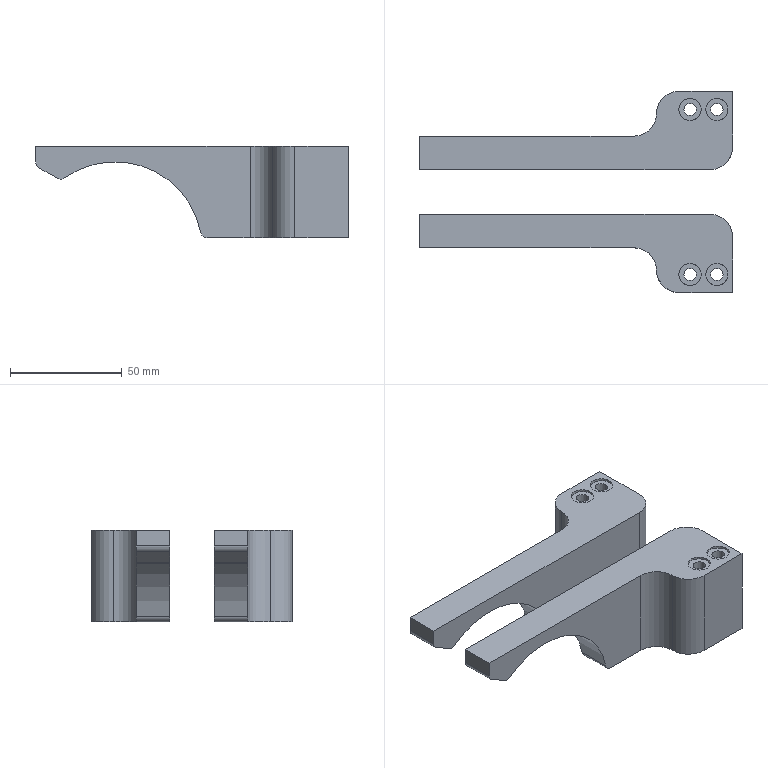Part | 2 solids | 50 faces | box 140 x 90 x 41 mm | volume 149726 mm3 | plane 26 | cylinder 24 | commonest cylinder face diameters 6 x6 20 x6 5.5 x4 10 x4 12.2 x2 78 x2
STEP:
#1=CARTESIAN_POINT('',(-68.5,-52.5,-9.64));
#2=VERTEX_POINT('',#1);
#3=CARTESIAN_POINT('',(-68.5,-37.5,-9.64));
#4=VERTEX_POINT('',#3);
#5=CARTESIAN_POINT('',(-68.5,-72.5,-9.64));
#6=DIRECTION('',(0.,1.,0.));
#7=VECTOR('',#6,1000.);
#8=LINE('',#5,#7);
#9=EDGE_CURVE('',#2,#4,#8,.T.);
#10=ORIENTED_EDGE('',*,*,#9,.F.);
#11=CARTESIAN_POINT('',(-70.,-52.5,-7.041));
#12=VERTEX_POINT('',#11);
#13=CARTESIAN_POINT('',(-67.,-52.5,-7.041));
#14=DIRECTION('',(0.,1.,0.));
#15=DIRECTION('',(-1.,0.,0.));
#16=AXIS2_PLACEMENT_3D('',#13,#14,#15);
#17=CIRCLE('',#16,3.);
#18=EDGE_CURVE('',#2,#12,#17,.T.);
#19=ORIENTED_EDGE('',*,*,#18,.T.);
#20=CARTESIAN_POINT('',(-70.,-37.5,-7.041));
#21=VERTEX_POINT('',#20);
#22=CARTESIAN_POINT('',(-70.,-72.5,-7.041));
#23=DIRECTION('',(0.,1.,0.));
#24=VECTOR('',#23,1000.);
#25=LINE('',#22,#24);
#26=EDGE_CURVE('',#12,#21,#25,.T.);
#27=ORIENTED_EDGE('',*,*,#26,.T.);
#28=CARTESIAN_POINT('',(-67.,-37.5,-7.041));
#29=DIRECTION('',(0.,-1.,0.));
#30=DIRECTION('',(1.,0.,0.));
#31=AXIS2_PLACEMENT_3D('',#28,#29,#30);
#32=CIRCLE('',#31,3.);
#33=EDGE_CURVE('',#21,#4,#32,.T.);
#34=ORIENTED_EDGE('',*,*,#33,.T.);
#35=EDGE_LOOP('',(#10,#19,#27,#34));
#36=FACE_BOUND('',#35,.T.);
#37=CARTESIAN_POINT('',(-67.,-72.5,-7.041));
#38=DIRECTION('',(0.,1.,0.));
#39=DIRECTION('',(-1.,0.,0.));
#40=AXIS2_PLACEMENT_3D('',#37,#38,#39);
#41=CYLINDRICAL_SURFACE('',#40,3.);
#42=ADVANCED_FACE('',(#36),#41,.T.);
#43=CARTESIAN_POINT('',(-60.27,-52.5,-14.391));
#44=VERTEX_POINT('',#43);
#45=CARTESIAN_POINT('',(-60.27,-37.5,-14.391));
#46=VERTEX_POINT('',#45);
#47=CARTESIAN_POINT('',(-60.27,-72.5,-14.391));
#48=DIRECTION('',(0.,1.,0.));
#49=VECTOR('',#48,1000.);
#50=LINE('',#47,#49);
#51=EDGE_CURVE('',#44,#46,#50,.T.);
#52=ORIENTED_EDGE('',*,*,#51,.F.);
#53=CARTESIAN_POINT('',(-68.5,-52.5,-9.64));
#54=DIRECTION('',(-0.866,0.,0.5));
#55=VECTOR('',#54,1000.);
#56=LINE('',#53,#55);
#57=EDGE_CURVE('',#44,#2,#56,.T.);
#58=ORIENTED_EDGE('',*,*,#57,.T.);
#59=ORIENTED_EDGE('',*,*,#9,.T.);
#60=CARTESIAN_POINT('',(-68.5,-37.5,-9.64));
#61=DIRECTION('',(0.866,0.,-0.5));
#62=VECTOR('',#61,1000.);
#63=LINE('',#60,#62);
#64=EDGE_CURVE('',#4,#46,#63,.T.);
#65=ORIENTED_EDGE('',*,*,#64,.T.);
#66=EDGE_LOOP('',(#52,#58,#59,#65));
#67=FACE_BOUND('',#66,.T.);
#68=CARTESIAN_POINT('',(-68.5,-72.5,-9.64));
#69=DIRECTION('',(0.5,0.,0.866));
#70=DIRECTION('',(-0.866,0.,0.5));
#71=AXIS2_PLACEMENT_3D('',#68,#69,#70);
#72=PLANE('',#71);
#73=ADVANCED_FACE('',(#67),#72,.F.);
#74=CARTESIAN_POINT('',(3.886,-52.5,-38.571));
#75=VERTEX_POINT('',#74);
#76=CARTESIAN_POINT('',(3.886,-37.5,-38.571));
#77=VERTEX_POINT('',#76);
#78=CARTESIAN_POINT('',(3.886,-72.5,-38.571));
#79=DIRECTION('',(0.,1.,0.));
#80=VECTOR('',#79,1000.);
#81=LINE('',#78,#80);
#82=EDGE_CURVE('',#75,#77,#81,.T.);
#83=ORIENTED_EDGE('',*,*,#82,.F.);
#84=CARTESIAN_POINT('',(-57.029,-52.5,-14.236));
#85=VERTEX_POINT('',#84);
#86=CARTESIAN_POINT('',(-34.4,-52.5,-46.));
#87=DIRECTION('',(0.,1.,0.));
#88=DIRECTION('',(-1.,0.,0.));
#89=AXIS2_PLACEMENT_3D('',#86,#87,#88);
#90=CIRCLE('',#89,39.);
#91=EDGE_CURVE('',#75,#85,#90,.F.);
#92=ORIENTED_EDGE('',*,*,#91,.T.);
#93=CARTESIAN_POINT('',(-57.029,-37.5,-14.236));
#94=VERTEX_POINT('',#93);
#95=CARTESIAN_POINT('',(-57.029,-72.5,-14.236));
#96=DIRECTION('',(0.,1.,0.));
#97=VECTOR('',#96,1000.);
#98=LINE('',#95,#97);
#99=EDGE_CURVE('',#85,#94,#98,.T.);
#100=ORIENTED_EDGE('',*,*,#99,.T.);
#101=CARTESIAN_POINT('',(-34.4,-37.5,-46.));
#102=DIRECTION('',(0.,1.,0.));
#103=DIRECTION('',(1.,0.,0.));
#104=AXIS2_PLACEMENT_3D('',#101,#102,#103);
#105=CIRCLE('',#104,39.);
#106=EDGE_CURVE('',#94,#77,#105,.T.);
#107=ORIENTED_EDGE('',*,*,#106,.T.);
#108=EDGE_LOOP('',(#83,#92,#100,#107));
#109=FACE_BOUND('',#108,.T.);
#110=CARTESIAN_POINT('',(-34.4,-72.5,-46.));
#111=DIRECTION('',(0.,1.,0.));
#112=DIRECTION('',(-1.,0.,0.));
#113=AXIS2_PLACEMENT_3D('',#110,#111,#112);
#114=CYLINDRICAL_SURFACE('',#113,39.);
#115=ADVANCED_FACE('',(#109),#114,.F.);
#116=ORIENTED_EDGE('',*,*,#99,.F.);
#117=CARTESIAN_POINT('',(-58.77,-52.5,-11.793));
#118=DIRECTION('',(0.,1.,0.));
#119=DIRECTION('',(-1.,0.,0.));
#120=AXIS2_PLACEMENT_3D('',#117,#118,#119);
#121=CIRCLE('',#120,3.);
#122=EDGE_CURVE('',#85,#44,#121,.T.);
#123=ORIENTED_EDGE('',*,*,#122,.T.);
#124=ORIENTED_EDGE('',*,*,#51,.T.);
#125=CARTESIAN_POINT('',(-58.77,-37.5,-11.793));
#126=DIRECTION('',(0.,-1.,0.));
#127=DIRECTION('',(1.,0.,0.));
#128=AXIS2_PLACEMENT_3D('',#125,#126,#127);
#129=CIRCLE('',#128,3.);
#130=EDGE_CURVE('',#46,#94,#129,.T.);
#131=ORIENTED_EDGE('',*,*,#130,.T.);
#132=EDGE_LOOP('',(#116,#123,#124,#131));
#133=FACE_BOUND('',#132,.T.);
#134=CARTESIAN_POINT('',(-58.77,-72.5,-11.793));
#135=DIRECTION('',(0.,1.,0.));
#136=DIRECTION('',(-1.,0.,0.));
#137=AXIS2_PLACEMENT_3D('',#134,#135,#136);
#138=CYLINDRICAL_SURFACE('',#137,3.);
#139=ADVANCED_FACE('',(#133),#138,.T.);
#140=CARTESIAN_POINT('',(6.831,-52.5,-41.));
#141=VERTEX_POINT('',#140);
#142=CARTESIAN_POINT('',(6.831,-37.5,-41.));
#143=VERTEX_POINT('',#142);
#144=CARTESIAN_POINT('',(6.831,-72.5,-41.));
#145=DIRECTION('',(0.,1.,0.));
#146=VECTOR('',#145,1000.);
#147=LINE('',#144,#146);
#148=EDGE_CURVE('',#141,#143,#147,.T.);
#149=ORIENTED_EDGE('',*,*,#148,.F.);
#150=CARTESIAN_POINT('',(6.831,-52.5,-38.));
#151=DIRECTION('',(0.,1.,0.));
#152=DIRECTION('',(-1.,0.,0.));
#153=AXIS2_PLACEMENT_3D('',#150,#151,#152);
#154=CIRCLE('',#153,3.);
#155=EDGE_CURVE('',#141,#75,#154,.T.);
#156=ORIENTED_EDGE('',*,*,#155,.T.);
#157=ORIENTED_EDGE('',*,*,#82,.T.);
#158=CARTESIAN_POINT('',(6.831,-37.5,-38.));
#159=DIRECTION('',(0.,-1.,0.));
#160=DIRECTION('',(1.,0.,0.));
#161=AXIS2_PLACEMENT_3D('',#158,#159,#160);
#162=CIRCLE('',#161,3.);
#163=EDGE_CURVE('',#77,#143,#162,.T.);
#164=ORIENTED_EDGE('',*,*,#163,.T.);
#165=EDGE_LOOP('',(#149,#156,#157,#164));
#166=FACE_BOUND('',#165,.T.);
#167=CARTESIAN_POINT('',(6.831,-72.5,-38.));
#168=DIRECTION('',(0.,1.,0.));
#169=DIRECTION('',(-1.,0.,0.));
#170=AXIS2_PLACEMENT_3D('',#167,#168,#169);
#171=CYLINDRICAL_SURFACE('',#170,3.);
#172=ADVANCED_FACE('',(#166),#171,.T.);
#173=CARTESIAN_POINT('',(36.,-62.5,-41.));
#174=VERTEX_POINT('',#173);
#175=CARTESIAN_POINT('',(46.,-72.5,-41.));
#176=VERTEX_POINT('',#175);
#177=CARTESIAN_POINT('',(46.,-62.5,-41.));
#178=DIRECTION('',(0.,0.,1.));
#179=DIRECTION('',(1.,0.,0.));
#180=AXIS2_PLACEMENT_3D('',#177,#178,#179);
#181=CIRCLE('',#180,10.);
#182=EDGE_CURVE('',#174,#176,#181,.T.);
#183=ORIENTED_EDGE('',*,*,#182,.T.);
#184=CARTESIAN_POINT('',(46.,-72.5,0.));
#185=VERTEX_POINT('',#184);
#186=CARTESIAN_POINT('',(46.,-72.5,0.));
#187=DIRECTION('',(0.,0.,-1.));
#188=VECTOR('',#187,1000.);
#189=LINE('',#186,#188);
#190=EDGE_CURVE('',#185,#176,#189,.T.);
#191=ORIENTED_EDGE('',*,*,#190,.F.);
#192=CARTESIAN_POINT('',(36.,-62.5,0.));
#193=VERTEX_POINT('',#192);
#194=CARTESIAN_POINT('',(46.,-62.5,0.));
#195=DIRECTION('',(0.,0.,1.));
#196=DIRECTION('',(1.,0.,0.));
#197=AXIS2_PLACEMENT_3D('',#194,#195,#196);
#198=CIRCLE('',#197,10.);
#199=EDGE_CURVE('',#193,#185,#198,.T.);
#200=ORIENTED_EDGE('',*,*,#199,.F.);
#201=CARTESIAN_POINT('',(36.,-62.5,0.));
#202=DIRECTION('',(0.,0.,-1.));
#203=VECTOR('',#202,1000.);
#204=LINE('',#201,#203);
#205=EDGE_CURVE('',#193,#174,#204,.T.);
#206=ORIENTED_EDGE('',*,*,#205,.T.);
#207=EDGE_LOOP('',(#183,#191,#200,#206));
#208=FACE_BOUND('',#207,.T.);
#209=CARTESIAN_POINT('',(46.,-62.5,0.));
#210=DIRECTION('',(0.,0.,-1.));
#211=DIRECTION('',(1.,0.,0.));
#212=AXIS2_PLACEMENT_3D('',#209,#210,#211);
#213=CYLINDRICAL_SURFACE('',#212,10.);
#214=ADVANCED_FACE('',(#208),#213,.T.);
#215=CARTESIAN_POINT('',(26.,-52.5,-41.));
#216=VERTEX_POINT('',#215);
#217=CARTESIAN_POINT('',(26.,-62.5,-41.));
#218=DIRECTION('',(0.,0.,1.));
#219=DIRECTION('',(0.,-1.,0.));
#220=AXIS2_PLACEMENT_3D('',#217,#218,#219);
#221=CIRCLE('',#220,10.);
#222=EDGE_CURVE('',#216,#174,#221,.F.);
#223=ORIENTED_EDGE('',*,*,#222,.T.);
#224=ORIENTED_EDGE('',*,*,#205,.F.);
#225=CARTESIAN_POINT('',(26.,-52.5,0.));
#226=VERTEX_POINT('',#225);
#227=CARTESIAN_POINT('',(26.,-62.5,0.));
#228=DIRECTION('',(0.,0.,-1.));
#229=DIRECTION('',(0.,1.,0.));
#230=AXIS2_PLACEMENT_3D('',#227,#228,#229);
#231=CIRCLE('',#230,10.);
#232=EDGE_CURVE('',#226,#193,#231,.T.);
#233=ORIENTED_EDGE('',*,*,#232,.F.);
#234=CARTESIAN_POINT('',(26.,-52.5,0.));
#235=DIRECTION('',(0.,0.,-1.));
#236=VECTOR('',#235,1000.);
#237=LINE('',#234,#236);
#238=EDGE_CURVE('',#226,#216,#237,.T.);
#239=ORIENTED_EDGE('',*,*,#238,.T.);
#240=EDGE_LOOP('',(#223,#224,#233,#239));
#241=FACE_BOUND('',#240,.T.);
#242=CARTESIAN_POINT('',(26.,-62.5,0.));
#243=DIRECTION('',(0.,0.,-1.));
#244=DIRECTION('',(1.,0.,0.));
#245=AXIS2_PLACEMENT_3D('',#242,#243,#244);
#246=CYLINDRICAL_SURFACE('',#245,10.);
#247=ADVANCED_FACE('',(#241),#246,.F.);
#248=ORIENTED_EDGE('',*,*,#155,.F.);
#249=CARTESIAN_POINT('',(-60.27,-52.5,-41.));
#250=DIRECTION('',(1.,0.,0.));
#251=VECTOR('',#250,1000.);
#252=LINE('',#249,#251);
#253=EDGE_CURVE('',#141,#216,#252,.T.);
#254=ORIENTED_EDGE('',*,*,#253,.T.);
#255=ORIENTED_EDGE('',*,*,#238,.F.);
#256=CARTESIAN_POINT('',(-70.,-52.5,0.));
#257=VERTEX_POINT('',#256);
#258=CARTESIAN_POINT('',(-57.029,-52.5,0.));
#259=DIRECTION('',(1.,0.,0.));
#260=VECTOR('',#259,1000.);
#261=LINE('',#258,#260);
#262=EDGE_CURVE('',#257,#226,#261,.T.);
#263=ORIENTED_EDGE('',*,*,#262,.F.);
#264=CARTESIAN_POINT('',(-70.,-52.5,0.));
#265=DIRECTION('',(0.,0.,-1.));
#266=VECTOR('',#265,1000.);
#267=LINE('',#264,#266);
#268=EDGE_CURVE('',#257,#12,#267,.T.);
#269=ORIENTED_EDGE('',*,*,#268,.T.);
#270=ORIENTED_EDGE('',*,*,#18,.F.);
#271=ORIENTED_EDGE('',*,*,#57,.F.);
#272=ORIENTED_EDGE('',*,*,#122,.F.);
#273=ORIENTED_EDGE('',*,*,#91,.F.);
#274=EDGE_LOOP('',(#248,#254,#255,#263,#269,#270,#271,#272,#273));
#275=FACE_BOUND('',#274,.T.);
#276=CARTESIAN_POINT('',(-60.27,-52.5,0.));
#277=DIRECTION('',(0.,1.,0.));
#278=DIRECTION('',(0.,0.,1.));
#279=AXIS2_PLACEMENT_3D('',#276,#277,#278);
#280=PLANE('',#279);
#281=ADVANCED_FACE('',(#275),#280,.F.);
#282=CARTESIAN_POINT('',(70.,-47.5,-41.));
#283=VERTEX_POINT('',#282);
#284=CARTESIAN_POINT('',(60.,-37.5,-41.));
#285=VERTEX_POINT('',#284);
#286=CARTESIAN_POINT('',(60.,-47.5,-41.));
#287=DIRECTION('',(0.,0.,1.));
#288=DIRECTION('',(1.,0.,0.));
#289=AXIS2_PLACEMENT_3D('',#286,#287,#288);
#290=CIRCLE('',#289,10.);
#291=EDGE_CURVE('',#283,#285,#290,.T.);
#292=ORIENTED_EDGE('',*,*,#291,.T.);
#293=CARTESIAN_POINT('',(60.,-37.5,0.));
#294=VERTEX_POINT('',#293);
#295=CARTESIAN_POINT('',(60.,-37.5,0.));
#296=DIRECTION('',(0.,0.,-1.));
#297=VECTOR('',#296,1000.);
#298=LINE('',#295,#297);
#299=EDGE_CURVE('',#294,#285,#298,.T.);
#300=ORIENTED_EDGE('',*,*,#299,.F.);
#301=CARTESIAN_POINT('',(70.,-47.5,0.));
#302=VERTEX_POINT('',#301);
#303=CARTESIAN_POINT('',(60.,-47.5,0.));
#304=DIRECTION('',(0.,0.,1.));
#305=DIRECTION('',(1.,0.,0.));
#306=AXIS2_PLACEMENT_3D('',#303,#304,#305);
#307=CIRCLE('',#306,10.);
#308=EDGE_CURVE('',#302,#294,#307,.T.);
#309=ORIENTED_EDGE('',*,*,#308,.F.);
#310=CARTESIAN_POINT('',(70.,-47.5,0.));
#311=DIRECTION('',(0.,0.,-1.));
#312=VECTOR('',#311,1000.);
#313=LINE('',#310,#312);
#314=EDGE_CURVE('',#302,#283,#313,.T.);
#315=ORIENTED_EDGE('',*,*,#314,.T.);
#316=EDGE_LOOP('',(#292,#300,#309,#315));
#317=FACE_BOUND('',#316,.T.);
#318=CARTESIAN_POINT('',(60.,-47.5,0.));
#319=DIRECTION('',(0.,0.,-1.));
#320=DIRECTION('',(1.,0.,0.));
#321=AXIS2_PLACEMENT_3D('',#318,#319,#320);
#322=CYLINDRICAL_SURFACE('',#321,10.);
#323=ADVANCED_FACE('',(#317),#322,.T.);
#324=CARTESIAN_POINT('',(65.753,-64.4,-1.));
#325=VERTEX_POINT('',#324);
#326=CARTESIAN_POINT('',(63.003,-64.4,-1.));
#327=DIRECTION('',(0.,0.,-1.));
#328=DIRECTION('',(1.,0.,0.));
#329=AXIS2_PLACEMENT_3D('',#326,#327,#328);
#330=CIRCLE('',#329,2.75);
#331=EDGE_CURVE('',#325,#325,#330,.F.);
#332=ORIENTED_EDGE('',*,*,#331,.T.);
#333=EDGE_LOOP('',(#332));
#334=FACE_BOUND('',#333,.T.);
#335=CARTESIAN_POINT('',(60.253,-64.4,-25.8));
#336=VERTEX_POINT('',#335);
#337=CARTESIAN_POINT('',(63.003,-64.4,-25.8));
#338=DIRECTION('',(0.,0.,1.));
#339=DIRECTION('',(-1.,0.,0.));
#340=AXIS2_PLACEMENT_3D('',#337,#338,#339);
#341=CIRCLE('',#340,2.75);
#342=EDGE_CURVE('',#336,#336,#341,.F.);
#343=ORIENTED_EDGE('',*,*,#342,.T.);
#344=EDGE_LOOP('',(#343));
#345=FACE_BOUND('',#344,.T.);
#346=CARTESIAN_POINT('',(63.003,-64.4,0.));
#347=DIRECTION('',(0.,0.,-1.));
#348=DIRECTION('',(1.,0.,0.));
#349=AXIS2_PLACEMENT_3D('',#346,#347,#348);
#350=CYLINDRICAL_SURFACE('',#349,2.75);
#351=ADVANCED_FACE('',(#334,#345),#350,.F.);
#352=CARTESIAN_POINT('',(44.9,-58.3,-41.));
#353=VERTEX_POINT('',#352);
#354=CARTESIAN_POINT('',(44.9,-70.5,-41.));
#355=VERTEX_POINT('',#354);
#356=CARTESIAN_POINT('',(44.9,-64.4,-41.));
#357=DIRECTION('',(0.,0.,1.));
#358=DIRECTION('',(0.,-1.,0.));
#359=AXIS2_PLACEMENT_3D('',#356,#357,#358);
#360=CIRCLE('',#359,6.1);
#361=EDGE_CURVE('',#353,#355,#360,.T.);
#362=ORIENTED_EDGE('',*,*,#361,.F.);
#363=CARTESIAN_POINT('',(44.9,-58.3,-25.8));
#364=VERTEX_POINT('',#363);
#365=CARTESIAN_POINT('',(44.9,-58.3,-25.8));
#366=DIRECTION('',(0.,0.,-1.));
#367=VECTOR('',#366,1000.);
#368=LINE('',#365,#367);
#369=EDGE_CURVE('',#353,#364,#368,.F.);
#370=ORIENTED_EDGE('',*,*,#369,.T.);
#371=CARTESIAN_POINT('',(44.9,-70.5,-25.8));
#372=VERTEX_POINT('',#371);
#373=CARTESIAN_POINT('',(44.9,-64.4,-25.8));
#374=DIRECTION('',(0.,0.,1.));
#375=DIRECTION('',(1.,0.,0.));
#376=AXIS2_PLACEMENT_3D('',#373,#374,#375);
#377=CIRCLE('',#376,6.1);
#378=EDGE_CURVE('',#372,#364,#377,.F.);
#379=ORIENTED_EDGE('',*,*,#378,.F.);
#380=CARTESIAN_POINT('',(44.9,-70.5,-25.8));
#381=DIRECTION('',(0.,0.,-1.));
#382=VECTOR('',#381,1000.);
#383=LINE('',#380,#382);
#384=EDGE_CURVE('',#355,#372,#383,.F.);
#385=ORIENTED_EDGE('',*,*,#384,.F.);
#386=EDGE_LOOP('',(#362,#370,#379,#385));
#387=FACE_BOUND('',#386,.T.);
#388=CARTESIAN_POINT('',(44.9,-64.4,-25.8));
#389=DIRECTION('',(0.,0.,-1.));
#390=DIRECTION('',(1.,0.,0.));
#391=AXIS2_PLACEMENT_3D('',#388,#389,#390);
#392=CYLINDRICAL_SURFACE('',#391,6.1);
#393=ADVANCED_FACE('',(#387),#392,.F.);
#394=CARTESIAN_POINT('',(70.,-70.5,-41.));
#395=VERTEX_POINT('',#394);
#396=CARTESIAN_POINT('',(44.9,-70.5,-41.));
#397=DIRECTION('',(1.,0.,0.));
#398=VECTOR('',#397,1000.);
#399=LINE('',#396,#398);
#400=EDGE_CURVE('',#355,#395,#399,.T.);
#401=ORIENTED_EDGE('',*,*,#400,.F.);
#402=ORIENTED_EDGE('',*,*,#384,.T.);
#403=CARTESIAN_POINT('',(70.,-70.5,-25.8));
#404=VERTEX_POINT('',#403);
#405=CARTESIAN_POINT('',(44.9,-70.5,-25.8));
#406=DIRECTION('',(1.,0.,0.));
#407=VECTOR('',#406,1000.);
#408=LINE('',#405,#407);
#409=EDGE_CURVE('',#404,#372,#408,.F.);
#410=ORIENTED_EDGE('',*,*,#409,.F.);
#411=CARTESIAN_POINT('',(70.,-70.5,-25.8));
#412=DIRECTION('',(0.,0.,-1.));
#413=VECTOR('',#412,1000.);
#414=LINE('',#411,#413);
#415=EDGE_CURVE('',#404,#395,#414,.T.);
#416=ORIENTED_EDGE('',*,*,#415,.T.);
#417=EDGE_LOOP('',(#401,#402,#410,#416));
#418=FACE_BOUND('',#417,.T.);
#419=CARTESIAN_POINT('',(44.9,-70.5,-25.8));
#420=DIRECTION('',(0.,1.,0.));
#421=DIRECTION('',(0.,0.,1.));
#422=AXIS2_PLACEMENT_3D('',#419,#420,#421);
#423=PLANE('',#422);
#424=ADVANCED_FACE('',(#418),#423,.T.);
#425=CARTESIAN_POINT('',(70.,-58.3,-41.));
#426=VERTEX_POINT('',#425);
#427=CARTESIAN_POINT('',(70.,-58.3,-41.));
#428=DIRECTION('',(-1.,0.,0.));
#429=VECTOR('',#428,1000.);
#430=LINE('',#427,#429);
#431=EDGE_CURVE('',#426,#353,#430,.T.);
#432=ORIENTED_EDGE('',*,*,#431,.F.);
#433=CARTESIAN_POINT('',(70.,-58.3,-25.8));
#434=VERTEX_POINT('',#433);
#435=CARTESIAN_POINT('',(70.,-58.3,-25.8));
#436=DIRECTION('',(0.,0.,-1.));
#437=VECTOR('',#436,1000.);
#438=LINE('',#435,#437);
#439=EDGE_CURVE('',#434,#426,#438,.T.);
#440=ORIENTED_EDGE('',*,*,#439,.F.);
#441=CARTESIAN_POINT('',(70.,-58.3,-25.8));
#442=DIRECTION('',(-1.,0.,0.));
#443=VECTOR('',#442,1000.);
#444=LINE('',#441,#443);
#445=EDGE_CURVE('',#364,#434,#444,.F.);
#446=ORIENTED_EDGE('',*,*,#445,.F.);
#447=ORIENTED_EDGE('',*,*,#369,.F.);
#448=EDGE_LOOP('',(#432,#440,#446,#447));
#449=FACE_BOUND('',#448,.T.);
#450=CARTESIAN_POINT('',(70.,-58.3,-25.8));
#451=DIRECTION('',(0.,-1.,0.));
#452=DIRECTION('',(0.,0.,-1.));
#453=AXIS2_PLACEMENT_3D('',#450,#451,#452);
#454=PLANE('',#453);
#455=ADVANCED_FACE('',(#449),#454,.T.);
#456=CARTESIAN_POINT('',(53.753,-64.4,-1.));
#457=VERTEX_POINT('',#456);
#458=CARTESIAN_POINT('',(51.003,-64.4,-1.));
#459=DIRECTION('',(0.,0.,-1.));
#460=DIRECTION('',(1.,0.,0.));
#461=AXIS2_PLACEMENT_3D('',#458,#459,#460);
#462=CIRCLE('',#461,2.75);
#463=EDGE_CURVE('',#457,#457,#462,.F.);
#464=ORIENTED_EDGE('',*,*,#463,.T.);
#465=EDGE_LOOP('',(#464));
#466=FACE_BOUND('',#465,.T.);
#467=CARTESIAN_POINT('',(48.253,-64.4,-25.8));
#468=VERTEX_POINT('',#467);
#469=CARTESIAN_POINT('',(51.003,-64.4,-25.8));
#470=DIRECTION('',(0.,0.,1.));
#471=DIRECTION('',(-1.,0.,0.));
#472=AXIS2_PLACEMENT_3D('',#469,#470,#471);
#473=CIRCLE('',#472,2.75);
#474=EDGE_CURVE('',#468,#468,#473,.F.);
#475=ORIENTED_EDGE('',*,*,#474,.T.);
#476=EDGE_LOOP('',(#475));
#477=FACE_BOUND('',#476,.T.);
#478=CARTESIAN_POINT('',(51.003,-64.4,0.));
#479=DIRECTION('',(0.,0.,-1.));
#480=DIRECTION('',(1.,0.,0.));
#481=AXIS2_PLACEMENT_3D('',#478,#479,#480);
#482=CYLINDRICAL_SURFACE('',#481,2.75);
#483=ADVANCED_FACE('',(#466,#477),#482,.F.);
#484=ORIENTED_EDGE('',*,*,#474,.F.);
#485=EDGE_LOOP('',(#484));
#486=FACE_BOUND('',#485,.T.);
#487=ORIENTED_EDGE('',*,*,#445,.T.);
#488=CARTESIAN_POINT('',(70.,-72.5,-25.8));
#489=DIRECTION('',(0.,1.,0.));
#490=VECTOR('',#489,1000.);
#491=LINE('',#488,#490);
#492=EDGE_CURVE('',#404,#434,#491,.T.);
#493=ORIENTED_EDGE('',*,*,#492,.F.);
#494=ORIENTED_EDGE('',*,*,#409,.T.);
#495=ORIENTED_EDGE('',*,*,#378,.T.);
#496=EDGE_LOOP('',(#487,#493,#494,#495));
#497=FACE_BOUND('',#496,.T.);
#498=ORIENTED_EDGE('',*,*,#342,.F.);
#499=EDGE_LOOP('',(#498));
#500=FACE_BOUND('',#499,.T.);
#501=CARTESIAN_POINT('',(44.9,-64.4,-25.8));
#502=DIRECTION('',(0.,0.,1.));
#503=DIRECTION('',(-1.,0.,0.));
#504=AXIS2_PLACEMENT_3D('',#501,#502,#503);
#505=PLANE('',#504);
#506=ADVANCED_FACE('',(#486,#497,#500),#505,.F.);
#507=CARTESIAN_POINT('',(68.003,-64.4,-1.));
#508=VERTEX_POINT('',#507);
#509=CARTESIAN_POINT('',(63.003,-64.4,-1.));
#510=DIRECTION('',(0.,0.,-1.));
#511=DIRECTION('',(1.,0.,0.));
#512=AXIS2_PLACEMENT_3D('',#509,#510,#511);
#513=CIRCLE('',#512,5.);
#514=EDGE_CURVE('',#508,#508,#513,.F.);
#515=ORIENTED_EDGE('',*,*,#514,.T.);
#516=EDGE_LOOP('',(#515));
#517=FACE_BOUND('',#516,.T.);
#518=ORIENTED_EDGE('',*,*,#331,.F.);
#519=EDGE_LOOP('',(#518));
#520=FACE_BOUND('',#519,.T.);
#521=CARTESIAN_POINT('',(63.003,-64.4,-1.));
#522=DIRECTION('',(0.,0.,-1.));
#523=DIRECTION('',(1.,0.,0.));
#524=AXIS2_PLACEMENT_3D('',#521,#522,#523);
#525=PLANE('',#524);
#526=ADVANCED_FACE('',(#517,#520),#525,.F.);
#527=ORIENTED_EDGE('',*,*,#514,.F.);
#528=EDGE_LOOP('',(#527));
#529=FACE_BOUND('',#528,.T.);
#530=CARTESIAN_POINT('',(63.003,-59.4,0.));
#531=VERTEX_POINT('',#530);
#532=CARTESIAN_POINT('',(63.003,-64.4,0.));
#533=DIRECTION('',(0.,0.,-1.));
#534=DIRECTION('',(0.,1.,0.));
#535=AXIS2_PLACEMENT_3D('',#532,#533,#534);
#536=CIRCLE('',#535,5.);
#537=EDGE_CURVE('',#531,#531,#536,.T.);
#538=ORIENTED_EDGE('',*,*,#537,.F.);
#539=EDGE_LOOP('',(#538));
#540=FACE_BOUND('',#539,.T.);
#541=CARTESIAN_POINT('',(63.003,-64.4,-1.));
#542=DIRECTION('',(0.,0.,1.));
#543=DIRECTION('',(-1.,0.,0.));
#544=AXIS2_PLACEMENT_3D('',#541,#542,#543);
#545=CYLINDRICAL_SURFACE('',#544,5.);
#546=ADVANCED_FACE('',(#529,#540),#545,.F.);
#547=CARTESIAN_POINT('',(56.003,-64.4,-1.));
#548=VERTEX_POINT('',#547);
#549=CARTESIAN_POINT('',(51.003,-64.4,-1.));
#550=DIRECTION('',(0.,0.,-1.));
#551=DIRECTION('',(1.,0.,0.));
#552=AXIS2_PLACEMENT_3D('',#549,#550,#551);
#553=CIRCLE('',#552,5.);
#554=EDGE_CURVE('',#548,#548,#553,.F.);
#555=ORIENTED_EDGE('',*,*,#554,.T.);
#556=EDGE_LOOP('',(#555));
#557=FACE_BOUND('',#556,.T.);
#558=ORIENTED_EDGE('',*,*,#463,.F.);
#559=EDGE_LOOP('',(#558));
#560=FACE_BOUND('',#559,.T.);
#561=CARTESIAN_POINT('',(51.003,-64.4,-1.));
#562=DIRECTION('',(0.,0.,-1.));
#563=DIRECTION('',(1.,0.,0.));
#564=AXIS2_PLACEMENT_3D('',#561,#562,#563);
#565=PLANE('',#564);
#566=ADVANCED_FACE('',(#557,#560),#565,.F.);
#567=ORIENTED_EDGE('',*,*,#554,.F.);
#568=EDGE_LOOP('',(#567));
#569=FACE_BOUND('',#568,.T.);
#570=CARTESIAN_POINT('',(51.003,-59.4,0.));
#571=VERTEX_POINT('',#570);
#572=CARTESIAN_POINT('',(51.003,-64.4,0.));
#573=DIRECTION('',(0.,0.,-1.));
#574=DIRECTION('',(0.,1.,0.));
#575=AXIS2_PLACEMENT_3D('',#572,#573,#574);
#576=CIRCLE('',#575,5.);
#577=EDGE_CURVE('',#571,#571,#576,.T.);
#578=ORIENTED_EDGE('',*,*,#577,.F.);
#579=EDGE_LOOP('',(#578));
#580=FACE_BOUND('',#579,.T.);
#581=CARTESIAN_POINT('',(51.003,-64.4,-1.));
#582=DIRECTION('',(0.,0.,1.));
#583=DIRECTION('',(-1.,0.,0.));
#584=AXIS2_PLACEMENT_3D('',#581,#582,#583);
#585=CYLINDRICAL_SURFACE('',#584,5.);
#586=ADVANCED_FACE('',(#569,#580),#585,.F.);
#587=ORIENTED_EDGE('',*,*,#314,.F.);
#588=CARTESIAN_POINT('',(70.,-72.5,0.));
#589=VERTEX_POINT('',#588);
#590=CARTESIAN_POINT('',(70.,-72.5,0.));
#591=DIRECTION('',(0.,1.,0.));
#592=VECTOR('',#591,1000.);
#593=LINE('',#590,#592);
#594=EDGE_CURVE('',#589,#302,#593,.T.);
#595=ORIENTED_EDGE('',*,*,#594,.F.);
#596=CARTESIAN_POINT('',(70.,-72.5,-41.));
#597=VERTEX_POINT('',#596);
#598=CARTESIAN_POINT('',(70.,-72.5,-41.));
#599=DIRECTION('',(0.,0.,1.));
#600=VECTOR('',#599,1000.);
#601=LINE('',#598,#600);
#602=EDGE_CURVE('',#589,#597,#601,.F.);
#603=ORIENTED_EDGE('',*,*,#602,.T.);
#604=CARTESIAN_POINT('',(70.,-72.5,-41.));
#605=DIRECTION('',(0.,1.,0.));
#606=VECTOR('',#605,1000.);
#607=LINE('',#604,#606);
#608=EDGE_CURVE('',#597,#395,#607,.T.);
#609=ORIENTED_EDGE('',*,*,#608,.T.);
#610=ORIENTED_EDGE('',*,*,#415,.F.);
#611=ORIENTED_EDGE('',*,*,#492,.T.);
#612=ORIENTED_EDGE('',*,*,#439,.T.);
#613=CARTESIAN_POINT('',(70.,-72.5,-41.));
#614=DIRECTION('',(0.,1.,0.));
#615=VECTOR('',#614,1000.);
#616=LINE('',#613,#615);
#617=EDGE_CURVE('',#426,#283,#616,.T.);
#618=ORIENTED_EDGE('',*,*,#617,.T.);
#619=EDGE_LOOP('',(#587,#595,#603,#609,#610,#611,#612,#618));
#620=FACE_BOUND('',#619,.T.);
#621=CARTESIAN_POINT('',(70.,-72.5,-41.));
#622=DIRECTION('',(-1.,0.,0.));
#623=DIRECTION('',(0.,-1.,0.));
#624=AXIS2_PLACEMENT_3D('',#621,#622,#623);
#625=PLANE('',#624);
#626=ADVANCED_FACE('',(#620),#625,.F.);
#627=ORIENTED_EDGE('',*,*,#617,.F.);
#628=ORIENTED_EDGE('',*,*,#431,.T.);
#629=ORIENTED_EDGE('',*,*,#361,.T.);
#630=ORIENTED_EDGE('',*,*,#400,.T.);
#631=ORIENTED_EDGE('',*,*,#608,.F.);
#632=CARTESIAN_POINT('',(6.831,-72.5,-41.));
#633=DIRECTION('',(1.,0.,0.));
#634=VECTOR('',#633,1000.);
#635=LINE('',#632,#634);
#636=EDGE_CURVE('',#176,#597,#635,.T.);
#637=ORIENTED_EDGE('',*,*,#636,.F.);
#638=ORIENTED_EDGE('',*,*,#182,.F.);
#639=ORIENTED_EDGE('',*,*,#222,.F.);
#640=ORIENTED_EDGE('',*,*,#253,.F.);
#641=ORIENTED_EDGE('',*,*,#148,.T.);
#642=CARTESIAN_POINT('',(46.,-37.5,-41.));
#643=DIRECTION('',(1.,0.,0.));
#644=VECTOR('',#643,1000.);
#645=LINE('',#642,#644);
#646=EDGE_CURVE('',#285,#143,#645,.F.);
#647=ORIENTED_EDGE('',*,*,#646,.F.);
#648=ORIENTED_EDGE('',*,*,#291,.F.);
#649=EDGE_LOOP('',(#627,#628,#629,#630,#631,#637,#638,#639,#640,#641,#647,#648));
#650=FACE_BOUND('',#649,.T.);
#651=CARTESIAN_POINT('',(46.,-72.5,-41.));
#652=DIRECTION('',(0.,0.,1.));
#653=DIRECTION('',(0.,-1.,0.));
#654=AXIS2_PLACEMENT_3D('',#651,#652,#653);
#655=PLANE('',#654);
#656=ADVANCED_FACE('',(#650),#655,.F.);
#657=ORIENTED_EDGE('',*,*,#577,.T.);
#658=EDGE_LOOP('',(#657));
#659=FACE_BOUND('',#658,.T.);
#660=ORIENTED_EDGE('',*,*,#537,.T.);
#661=EDGE_LOOP('',(#660));
#662=FACE_BOUND('',#661,.T.);
#663=CARTESIAN_POINT('',(-70.,-37.5,0.));
#664=VERTEX_POINT('',#663);
#665=CARTESIAN_POINT('',(-70.,-72.5,0.));
#666=DIRECTION('',(0.,1.,0.));
#667=VECTOR('',#666,1000.);
#668=LINE('',#665,#667);
#669=EDGE_CURVE('',#664,#257,#668,.F.);
#670=ORIENTED_EDGE('',*,*,#669,.T.);
#671=ORIENTED_EDGE('',*,*,#262,.T.);
#672=ORIENTED_EDGE('',*,*,#232,.T.);
#673=ORIENTED_EDGE('',*,*,#199,.T.);
#674=CARTESIAN_POINT('',(70.,-72.5,0.));
#675=DIRECTION('',(-1.,0.,0.));
#676=VECTOR('',#675,1000.);
#677=LINE('',#674,#676);
#678=EDGE_CURVE('',#185,#589,#677,.F.);
#679=ORIENTED_EDGE('',*,*,#678,.T.);
#680=ORIENTED_EDGE('',*,*,#594,.T.);
#681=ORIENTED_EDGE('',*,*,#308,.T.);
#682=CARTESIAN_POINT('',(-60.,-37.5,0.));
#683=DIRECTION('',(-1.,0.,0.));
#684=VECTOR('',#683,1000.);
#685=LINE('',#682,#684);
#686=EDGE_CURVE('',#294,#664,#685,.T.);
#687=ORIENTED_EDGE('',*,*,#686,.T.);
#688=EDGE_LOOP('',(#670,#671,#672,#673,#679,#680,#681,#687));
#689=FACE_BOUND('',#688,.T.);
#690=CARTESIAN_POINT('',(-60.,-72.5,0.));
#691=DIRECTION('',(0.,0.,-1.));
#692=DIRECTION('',(0.,1.,0.));
#693=AXIS2_PLACEMENT_3D('',#690,#691,#692);
#694=PLANE('',#693);
#695=ADVANCED_FACE('',(#659,#662,#689),#694,.F.);
#696=ORIENTED_EDGE('',*,*,#686,.F.);
#697=ORIENTED_EDGE('',*,*,#299,.T.);
#698=ORIENTED_EDGE('',*,*,#646,.T.);
#699=ORIENTED_EDGE('',*,*,#163,.F.);
#700=ORIENTED_EDGE('',*,*,#106,.F.);
#701=ORIENTED_EDGE('',*,*,#130,.F.);
#702=ORIENTED_EDGE('',*,*,#64,.F.);
#703=ORIENTED_EDGE('',*,*,#33,.F.);
#704=CARTESIAN_POINT('',(-70.,-37.5,0.));
#705=DIRECTION('',(0.,0.,-1.));
#706=VECTOR('',#705,1000.);
#707=LINE('',#704,#706);
#708=EDGE_CURVE('',#664,#21,#707,.T.);
#709=ORIENTED_EDGE('',*,*,#708,.F.);
#710=EDGE_LOOP('',(#696,#697,#698,#699,#700,#701,#702,#703,#709));
#711=FACE_BOUND('',#710,.T.);
#712=CARTESIAN_POINT('',(-34.4,-37.5,-46.));
#713=DIRECTION('',(0.,1.,0.));
#714=DIRECTION('',(-1.,0.,0.));
#715=AXIS2_PLACEMENT_3D('',#712,#713,#714);
#716=PLANE('',#715);
#717=ADVANCED_FACE('',(#711),#716,.T.);
#718=ORIENTED_EDGE('',*,*,#678,.F.);
#719=ORIENTED_EDGE('',*,*,#190,.T.);
#720=ORIENTED_EDGE('',*,*,#636,.T.);
#721=ORIENTED_EDGE('',*,*,#602,.F.);
#722=EDGE_LOOP('',(#718,#719,#720,#721));
#723=FACE_BOUND('',#722,.T.);
#724=CARTESIAN_POINT('',(-34.4,-72.5,-46.));
#725=DIRECTION('',(0.,1.,0.));
#726=DIRECTION('',(-1.,0.,0.));
#727=AXIS2_PLACEMENT_3D('',#724,#725,#726);
#728=PLANE('',#727);
#729=ADVANCED_FACE('',(#723),#728,.F.);
#730=ORIENTED_EDGE('',*,*,#268,.F.);
#731=ORIENTED_EDGE('',*,*,#669,.F.);
#732=ORIENTED_EDGE('',*,*,#708,.T.);
#733=ORIENTED_EDGE('',*,*,#26,.F.);
#734=EDGE_LOOP('',(#730,#731,#732,#733));
#735=FACE_BOUND('',#734,.T.);
#736=CARTESIAN_POINT('',(-70.,-72.5,0.));
#737=DIRECTION('',(1.,0.,0.));
#738=DIRECTION('',(0.,1.,0.));
#739=AXIS2_PLACEMENT_3D('',#736,#737,#738);
#740=PLANE('',#739);
#741=ADVANCED_FACE('',(#735),#740,.F.);
#742=CLOSED_SHELL('',(#42,#73,#115,#139,#172,#214,#247,#281,#323,#351,#393,#424,#455,#483,#506,#526,#546,#566,#586,#626,#656,#695,#717,#729,#741));
#743=MANIFOLD_SOLID_BREP('',#742);
#744=CARTESIAN_POINT('',(36.,7.5,-41.));
#745=VERTEX_POINT('',#744);
#746=CARTESIAN_POINT('',(46.,17.5,-41.));
#747=VERTEX_POINT('',#746);
#748=CARTESIAN_POINT('',(46.,7.5,-41.));
#749=DIRECTION('',(0.,0.,-1.));
#750=DIRECTION('',(1.,0.,0.));
#751=AXIS2_PLACEMENT_3D('',#748,#749,#750);
#752=CIRCLE('',#751,10.);
#753=EDGE_CURVE('',#745,#747,#752,.T.);
#754=ORIENTED_EDGE('',*,*,#753,.F.);
#755=CARTESIAN_POINT('',(36.,7.5,0.));
#756=VERTEX_POINT('',#755);
#757=CARTESIAN_POINT('',(36.,7.5,0.));
#758=DIRECTION('',(0.,0.,-1.));
#759=VECTOR('',#758,1000.);
#760=LINE('',#757,#759);
#761=EDGE_CURVE('',#756,#745,#760,.T.);
#762=ORIENTED_EDGE('',*,*,#761,.F.);
#763=CARTESIAN_POINT('',(46.,17.5,0.));
#764=VERTEX_POINT('',#763);
#765=CARTESIAN_POINT('',(46.,7.5,0.));
#766=DIRECTION('',(0.,0.,-1.));
#767=DIRECTION('',(1.,0.,0.));
#768=AXIS2_PLACEMENT_3D('',#765,#766,#767);
#769=CIRCLE('',#768,10.);
#770=EDGE_CURVE('',#756,#764,#769,.T.);
#771=ORIENTED_EDGE('',*,*,#770,.T.);
#772=CARTESIAN_POINT('',(46.,17.5,0.));
#773=DIRECTION('',(0.,0.,-1.));
#774=VECTOR('',#773,1000.);
#775=LINE('',#772,#774);
#776=EDGE_CURVE('',#764,#747,#775,.T.);
#777=ORIENTED_EDGE('',*,*,#776,.T.);
#778=EDGE_LOOP('',(#754,#762,#771,#777));
#779=FACE_BOUND('',#778,.T.);
#780=CARTESIAN_POINT('',(46.,7.5,0.));
#781=DIRECTION('',(0.,0.,-1.));
#782=DIRECTION('',(1.,0.,0.));
#783=AXIS2_PLACEMENT_3D('',#780,#781,#782);
#784=CYLINDRICAL_SURFACE('',#783,10.);
#785=ADVANCED_FACE('',(#779),#784,.T.);
#786=CARTESIAN_POINT('',(26.,-2.5,-41.));
#787=VERTEX_POINT('',#786);
#788=CARTESIAN_POINT('',(26.,7.5,-41.));
#789=DIRECTION('',(0.,0.,-1.));
#790=DIRECTION('',(0.,1.,0.));
#791=AXIS2_PLACEMENT_3D('',#788,#789,#790);
#792=CIRCLE('',#791,10.);
#793=EDGE_CURVE('',#787,#745,#792,.F.);
#794=ORIENTED_EDGE('',*,*,#793,.F.);
#795=CARTESIAN_POINT('',(26.,-2.5,0.));
#796=VERTEX_POINT('',#795);
#797=CARTESIAN_POINT('',(26.,-2.5,0.));
#798=DIRECTION('',(0.,0.,-1.));
#799=VECTOR('',#798,1000.);
#800=LINE('',#797,#799);
#801=EDGE_CURVE('',#796,#787,#800,.T.);
#802=ORIENTED_EDGE('',*,*,#801,.F.);
#803=CARTESIAN_POINT('',(26.,7.5,0.));
#804=DIRECTION('',(0.,0.,1.));
#805=DIRECTION('',(0.,-1.,0.));
#806=AXIS2_PLACEMENT_3D('',#803,#804,#805);
#807=CIRCLE('',#806,10.);
#808=EDGE_CURVE('',#796,#756,#807,.T.);
#809=ORIENTED_EDGE('',*,*,#808,.T.);
#810=ORIENTED_EDGE('',*,*,#761,.T.);
#811=EDGE_LOOP('',(#794,#802,#809,#810));
#812=FACE_BOUND('',#811,.T.);
#813=CARTESIAN_POINT('',(26.,7.5,0.));
#814=DIRECTION('',(0.,0.,-1.));
#815=DIRECTION('',(1.,0.,0.));
#816=AXIS2_PLACEMENT_3D('',#813,#814,#815);
#817=CYLINDRICAL_SURFACE('',#816,10.);
#818=ADVANCED_FACE('',(#812),#817,.F.);
#819=CARTESIAN_POINT('',(6.831,-2.5,-41.));
#820=VERTEX_POINT('',#819);
#821=CARTESIAN_POINT('',(3.886,-2.5,-38.571));
#822=VERTEX_POINT('',#821);
#823=CARTESIAN_POINT('',(6.831,-2.5,-38.));
#824=DIRECTION('',(0.,1.,0.));
#825=DIRECTION('',(-1.,0.,0.));
#826=AXIS2_PLACEMENT_3D('',#823,#824,#825);
#827=CIRCLE('',#826,3.);
#828=EDGE_CURVE('',#820,#822,#827,.T.);
#829=ORIENTED_EDGE('',*,*,#828,.T.);
#830=CARTESIAN_POINT('',(-57.029,-2.5,-14.236));
#831=VERTEX_POINT('',#830);
#832=CARTESIAN_POINT('',(-34.4,-2.5,-46.));
#833=DIRECTION('',(0.,1.,0.));
#834=DIRECTION('',(-1.,0.,0.));
#835=AXIS2_PLACEMENT_3D('',#832,#833,#834);
#836=CIRCLE('',#835,39.);
#837=EDGE_CURVE('',#822,#831,#836,.F.);
#838=ORIENTED_EDGE('',*,*,#837,.T.);
#839=CARTESIAN_POINT('',(-60.27,-2.5,-14.391));
#840=VERTEX_POINT('',#839);
#841=CARTESIAN_POINT('',(-58.77,-2.5,-11.793));
#842=DIRECTION('',(0.,1.,0.));
#843=DIRECTION('',(-1.,0.,0.));
#844=AXIS2_PLACEMENT_3D('',#841,#842,#843);
#845=CIRCLE('',#844,3.);
#846=EDGE_CURVE('',#831,#840,#845,.T.);
#847=ORIENTED_EDGE('',*,*,#846,.T.);
#848=CARTESIAN_POINT('',(-68.5,-2.5,-9.64));
#849=VERTEX_POINT('',#848);
#850=CARTESIAN_POINT('',(-68.5,-2.5,-9.64));
#851=DIRECTION('',(-0.866,0.,0.5));
#852=VECTOR('',#851,1000.);
#853=LINE('',#850,#852);
#854=EDGE_CURVE('',#840,#849,#853,.T.);
#855=ORIENTED_EDGE('',*,*,#854,.T.);
#856=CARTESIAN_POINT('',(-70.,-2.5,-7.041));
#857=VERTEX_POINT('',#856);
#858=CARTESIAN_POINT('',(-67.,-2.5,-7.041));
#859=DIRECTION('',(0.,1.,0.));
#860=DIRECTION('',(-1.,0.,0.));
#861=AXIS2_PLACEMENT_3D('',#858,#859,#860);
#862=CIRCLE('',#861,3.);
#863=EDGE_CURVE('',#849,#857,#862,.T.);
#864=ORIENTED_EDGE('',*,*,#863,.T.);
#865=CARTESIAN_POINT('',(-70.,-2.5,0.));
#866=VERTEX_POINT('',#865);
#867=CARTESIAN_POINT('',(-70.,-2.5,0.));
#868=DIRECTION('',(0.,0.,-1.));
#869=VECTOR('',#868,1000.);
#870=LINE('',#867,#869);
#871=EDGE_CURVE('',#866,#857,#870,.T.);
#872=ORIENTED_EDGE('',*,*,#871,.F.);
#873=CARTESIAN_POINT('',(-57.029,-2.5,0.));
#874=DIRECTION('',(1.,0.,0.));
#875=VECTOR('',#874,1000.);
#876=LINE('',#873,#875);
#877=EDGE_CURVE('',#866,#796,#876,.T.);
#878=ORIENTED_EDGE('',*,*,#877,.T.);
#879=ORIENTED_EDGE('',*,*,#801,.T.);
#880=CARTESIAN_POINT('',(-60.27,-2.5,-41.));
#881=DIRECTION('',(1.,0.,0.));
#882=VECTOR('',#881,1000.);
#883=LINE('',#880,#882);
#884=EDGE_CURVE('',#820,#787,#883,.T.);
#885=ORIENTED_EDGE('',*,*,#884,.F.);
#886=EDGE_LOOP('',(#829,#838,#847,#855,#864,#872,#878,#879,#885));
#887=FACE_BOUND('',#886,.T.);
#888=CARTESIAN_POINT('',(-60.27,-2.5,0.));
#889=DIRECTION('',(0.,-1.,0.));
#890=DIRECTION('',(0.,0.,1.));
#891=AXIS2_PLACEMENT_3D('',#888,#889,#890);
#892=PLANE('',#891);
#893=ADVANCED_FACE('',(#887),#892,.F.);
#894=CARTESIAN_POINT('',(-68.5,-17.5,-9.64));
#895=VERTEX_POINT('',#894);
#896=CARTESIAN_POINT('',(-68.5,17.5,-9.64));
#897=DIRECTION('',(0.,-1.,0.));
#898=VECTOR('',#897,1000.);
#899=LINE('',#896,#898);
#900=EDGE_CURVE('',#849,#895,#899,.T.);
#901=ORIENTED_EDGE('',*,*,#900,.T.);
#902=CARTESIAN_POINT('',(-70.,-17.5,-7.041));
#903=VERTEX_POINT('',#902);
#904=CARTESIAN_POINT('',(-67.,-17.5,-7.041));
#905=DIRECTION('',(0.,-1.,0.));
#906=DIRECTION('',(1.,0.,0.));
#907=AXIS2_PLACEMENT_3D('',#904,#905,#906);
#908=CIRCLE('',#907,3.);
#909=EDGE_CURVE('',#903,#895,#908,.T.);
#910=ORIENTED_EDGE('',*,*,#909,.F.);
#911=CARTESIAN_POINT('',(-70.,17.5,-7.041));
#912=DIRECTION('',(0.,-1.,0.));
#913=VECTOR('',#912,1000.);
#914=LINE('',#911,#913);
#915=EDGE_CURVE('',#857,#903,#914,.T.);
#916=ORIENTED_EDGE('',*,*,#915,.F.);
#917=ORIENTED_EDGE('',*,*,#863,.F.);
#918=EDGE_LOOP('',(#901,#910,#916,#917));
#919=FACE_BOUND('',#918,.T.);
#920=CARTESIAN_POINT('',(-67.,17.5,-7.041));
#921=DIRECTION('',(0.,-1.,0.));
#922=DIRECTION('',(-1.,0.,0.));
#923=AXIS2_PLACEMENT_3D('',#920,#921,#922);
#924=CYLINDRICAL_SURFACE('',#923,3.);
#925=ADVANCED_FACE('',(#919),#924,.T.);
#926=CARTESIAN_POINT('',(-60.27,-17.5,-14.391));
#927=VERTEX_POINT('',#926);
#928=CARTESIAN_POINT('',(-60.27,17.5,-14.391));
#929=DIRECTION('',(0.,-1.,0.));
#930=VECTOR('',#929,1000.);
#931=LINE('',#928,#930);
#932=EDGE_CURVE('',#840,#927,#931,.T.);
#933=ORIENTED_EDGE('',*,*,#932,.T.);
#934=CARTESIAN_POINT('',(-68.5,-17.5,-9.64));
#935=DIRECTION('',(0.866,0.,-0.5));
#936=VECTOR('',#935,1000.);
#937=LINE('',#934,#936);
#938=EDGE_CURVE('',#895,#927,#937,.T.);
#939=ORIENTED_EDGE('',*,*,#938,.F.);
#940=ORIENTED_EDGE('',*,*,#900,.F.);
#941=ORIENTED_EDGE('',*,*,#854,.F.);
#942=EDGE_LOOP('',(#933,#939,#940,#941));
#943=FACE_BOUND('',#942,.T.);
#944=CARTESIAN_POINT('',(-68.5,17.5,-9.64));
#945=DIRECTION('',(0.5,0.,0.866));
#946=DIRECTION('',(-0.866,0.,0.5));
#947=AXIS2_PLACEMENT_3D('',#944,#945,#946);
#948=PLANE('',#947);
#949=ADVANCED_FACE('',(#943),#948,.F.);
#950=CARTESIAN_POINT('',(3.886,-17.5,-38.571));
#951=VERTEX_POINT('',#950);
#952=CARTESIAN_POINT('',(3.886,17.5,-38.571));
#953=DIRECTION('',(0.,-1.,0.));
#954=VECTOR('',#953,1000.);
#955=LINE('',#952,#954);
#956=EDGE_CURVE('',#822,#951,#955,.T.);
#957=ORIENTED_EDGE('',*,*,#956,.T.);
#958=CARTESIAN_POINT('',(-57.029,-17.5,-14.236));
#959=VERTEX_POINT('',#958);
#960=CARTESIAN_POINT('',(-34.4,-17.5,-46.));
#961=DIRECTION('',(0.,1.,0.));
#962=DIRECTION('',(1.,0.,0.));
#963=AXIS2_PLACEMENT_3D('',#960,#961,#962);
#964=CIRCLE('',#963,39.);
#965=EDGE_CURVE('',#959,#951,#964,.T.);
#966=ORIENTED_EDGE('',*,*,#965,.F.);
#967=CARTESIAN_POINT('',(-57.029,17.5,-14.236));
#968=DIRECTION('',(0.,-1.,0.));
#969=VECTOR('',#968,1000.);
#970=LINE('',#967,#969);
#971=EDGE_CURVE('',#831,#959,#970,.T.);
#972=ORIENTED_EDGE('',*,*,#971,.F.);
#973=ORIENTED_EDGE('',*,*,#837,.F.);
#974=EDGE_LOOP('',(#957,#966,#972,#973));
#975=FACE_BOUND('',#974,.T.);
#976=CARTESIAN_POINT('',(-34.4,17.5,-46.));
#977=DIRECTION('',(0.,-1.,0.));
#978=DIRECTION('',(-1.,0.,0.));
#979=AXIS2_PLACEMENT_3D('',#976,#977,#978);
#980=CYLINDRICAL_SURFACE('',#979,39.);
#981=ADVANCED_FACE('',(#975),#980,.F.);
#982=ORIENTED_EDGE('',*,*,#971,.T.);
#983=CARTESIAN_POINT('',(-58.77,-17.5,-11.793));
#984=DIRECTION('',(0.,-1.,0.));
#985=DIRECTION('',(1.,0.,0.));
#986=AXIS2_PLACEMENT_3D('',#983,#984,#985);
#987=CIRCLE('',#986,3.);
#988=EDGE_CURVE('',#927,#959,#987,.T.);
#989=ORIENTED_EDGE('',*,*,#988,.F.);
#990=ORIENTED_EDGE('',*,*,#932,.F.);
#991=ORIENTED_EDGE('',*,*,#846,.F.);
#992=EDGE_LOOP('',(#982,#989,#990,#991));
#993=FACE_BOUND('',#992,.T.);
#994=CARTESIAN_POINT('',(-58.77,17.5,-11.793));
#995=DIRECTION('',(0.,-1.,0.));
#996=DIRECTION('',(-1.,0.,0.));
#997=AXIS2_PLACEMENT_3D('',#994,#995,#996);
#998=CYLINDRICAL_SURFACE('',#997,3.);
#999=ADVANCED_FACE('',(#993),#998,.T.);
#1000=CARTESIAN_POINT('',(6.831,-17.5,-41.));
#1001=VERTEX_POINT('',#1000);
#1002=CARTESIAN_POINT('',(6.831,17.5,-41.));
#1003=DIRECTION('',(0.,-1.,0.));
#1004=VECTOR('',#1003,1000.);
#1005=LINE('',#1002,#1004);
#1006=EDGE_CURVE('',#820,#1001,#1005,.T.);
#1007=ORIENTED_EDGE('',*,*,#1006,.T.);
#1008=CARTESIAN_POINT('',(6.831,-17.5,-38.));
#1009=DIRECTION('',(0.,-1.,0.));
#1010=DIRECTION('',(1.,0.,0.));
#1011=AXIS2_PLACEMENT_3D('',#1008,#1009,#1010);
#1012=CIRCLE('',#1011,3.);
#1013=EDGE_CURVE('',#951,#1001,#1012,.T.);
#1014=ORIENTED_EDGE('',*,*,#1013,.F.);
#1015=ORIENTED_EDGE('',*,*,#956,.F.);
#1016=ORIENTED_EDGE('',*,*,#828,.F.);
#1017=EDGE_LOOP('',(#1007,#1014,#1015,#1016));
#1018=FACE_BOUND('',#1017,.T.);
#1019=CARTESIAN_POINT('',(6.831,17.5,-38.));
#1020=DIRECTION('',(0.,-1.,0.));
#1021=DIRECTION('',(-1.,0.,0.));
#1022=AXIS2_PLACEMENT_3D('',#1019,#1020,#1021);
#1023=CYLINDRICAL_SURFACE('',#1022,3.);
#1024=ADVANCED_FACE('',(#1018),#1023,.T.);
#1025=CARTESIAN_POINT('',(60.,-17.5,0.));
#1026=VERTEX_POINT('',#1025);
#1027=CARTESIAN_POINT('',(-70.,-17.5,0.));
#1028=VERTEX_POINT('',#1027);
#1029=CARTESIAN_POINT('',(-60.,-17.5,0.));
#1030=DIRECTION('',(-1.,0.,0.));
#1031=VECTOR('',#1030,1000.);
#1032=LINE('',#1029,#1031);
#1033=EDGE_CURVE('',#1026,#1028,#1032,.T.);
#1034=ORIENTED_EDGE('',*,*,#1033,.T.);
#1035=CARTESIAN_POINT('',(-70.,-17.5,0.));
#1036=DIRECTION('',(0.,0.,-1.));
#1037=VECTOR('',#1036,1000.);
#1038=LINE('',#1035,#1037);
#1039=EDGE_CURVE('',#1028,#903,#1038,.T.);
#1040=ORIENTED_EDGE('',*,*,#1039,.T.);
#1041=ORIENTED_EDGE('',*,*,#909,.T.);
#1042=ORIENTED_EDGE('',*,*,#938,.T.);
#1043=ORIENTED_EDGE('',*,*,#988,.T.);
#1044=ORIENTED_EDGE('',*,*,#965,.T.);
#1045=ORIENTED_EDGE('',*,*,#1013,.T.);
#1046=CARTESIAN_POINT('',(60.,-17.5,-41.));
#1047=VERTEX_POINT('',#1046);
#1048=CARTESIAN_POINT('',(46.,-17.5,-41.));
#1049=DIRECTION('',(1.,0.,0.));
#1050=VECTOR('',#1049,1000.);
#1051=LINE('',#1048,#1050);
#1052=EDGE_CURVE('',#1047,#1001,#1051,.F.);
#1053=ORIENTED_EDGE('',*,*,#1052,.F.);
#1054=CARTESIAN_POINT('',(60.,-17.5,0.));
#1055=DIRECTION('',(0.,0.,-1.));
#1056=VECTOR('',#1055,1000.);
#1057=LINE('',#1054,#1056);
#1058=EDGE_CURVE('',#1026,#1047,#1057,.T.);
#1059=ORIENTED_EDGE('',*,*,#1058,.F.);
#1060=EDGE_LOOP('',(#1034,#1040,#1041,#1042,#1043,#1044,#1045,#1053,#1059));
#1061=FACE_BOUND('',#1060,.T.);
#1062=CARTESIAN_POINT('',(-34.4,-17.5,-46.));
#1063=DIRECTION('',(0.,-1.,0.));
#1064=DIRECTION('',(-1.,0.,0.));
#1065=AXIS2_PLACEMENT_3D('',#1062,#1063,#1064);
#1066=PLANE('',#1065);
#1067=ADVANCED_FACE('',(#1061),#1066,.T.);
#1068=CARTESIAN_POINT('',(51.003,4.4,0.));
#1069=VERTEX_POINT('',#1068);
#1070=CARTESIAN_POINT('',(51.003,9.4,0.));
#1071=DIRECTION('',(0.,0.,1.));
#1072=DIRECTION('',(0.,-1.,0.));
#1073=AXIS2_PLACEMENT_3D('',#1070,#1071,#1072);
#1074=CIRCLE('',#1073,5.);
#1075=EDGE_CURVE('',#1069,#1069,#1074,.T.);
#1076=ORIENTED_EDGE('',*,*,#1075,.F.);
#1077=EDGE_LOOP('',(#1076));
#1078=FACE_BOUND('',#1077,.T.);
#1079=CARTESIAN_POINT('',(63.003,4.4,0.));
#1080=VERTEX_POINT('',#1079);
#1081=CARTESIAN_POINT('',(63.003,9.4,0.));
#1082=DIRECTION('',(0.,0.,1.));
#1083=DIRECTION('',(0.,-1.,0.));
#1084=AXIS2_PLACEMENT_3D('',#1081,#1082,#1083);
#1085=CIRCLE('',#1084,5.);
#1086=EDGE_CURVE('',#1080,#1080,#1085,.T.);
#1087=ORIENTED_EDGE('',*,*,#1086,.F.);
#1088=EDGE_LOOP('',(#1087));
#1089=FACE_BOUND('',#1088,.T.);
#1090=CARTESIAN_POINT('',(-70.,17.5,0.));
#1091=DIRECTION('',(0.,-1.,0.));
#1092=VECTOR('',#1091,1000.);
#1093=LINE('',#1090,#1092);
#1094=EDGE_CURVE('',#1028,#866,#1093,.F.);
#1095=ORIENTED_EDGE('',*,*,#1094,.F.);
#1096=ORIENTED_EDGE('',*,*,#1033,.F.);
#1097=CARTESIAN_POINT('',(70.,-7.5,0.));
#1098=VERTEX_POINT('',#1097);
#1099=CARTESIAN_POINT('',(60.,-7.5,0.));
#1100=DIRECTION('',(0.,0.,-1.));
#1101=DIRECTION('',(1.,0.,0.));
#1102=AXIS2_PLACEMENT_3D('',#1099,#1100,#1101);
#1103=CIRCLE('',#1102,10.);
#1104=EDGE_CURVE('',#1098,#1026,#1103,.T.);
#1105=ORIENTED_EDGE('',*,*,#1104,.F.);
#1106=CARTESIAN_POINT('',(70.,17.5,0.));
#1107=VERTEX_POINT('',#1106);
#1108=CARTESIAN_POINT('',(70.,17.5,0.));
#1109=DIRECTION('',(0.,-1.,0.));
#1110=VECTOR('',#1109,1000.);
#1111=LINE('',#1108,#1110);
#1112=EDGE_CURVE('',#1107,#1098,#1111,.T.);
#1113=ORIENTED_EDGE('',*,*,#1112,.F.);
#1114=CARTESIAN_POINT('',(70.,17.5,0.));
#1115=DIRECTION('',(-1.,0.,0.));
#1116=VECTOR('',#1115,1000.);
#1117=LINE('',#1114,#1116);
#1118=EDGE_CURVE('',#764,#1107,#1117,.F.);
#1119=ORIENTED_EDGE('',*,*,#1118,.F.);
#1120=ORIENTED_EDGE('',*,*,#770,.F.);
#1121=ORIENTED_EDGE('',*,*,#808,.F.);
#1122=ORIENTED_EDGE('',*,*,#877,.F.);
#1123=EDGE_LOOP('',(#1095,#1096,#1105,#1113,#1119,#1120,#1121,#1122));
#1124=FACE_BOUND('',#1123,.T.);
#1125=CARTESIAN_POINT('',(-60.,17.5,0.));
#1126=DIRECTION('',(0.,0.,-1.));
#1127=DIRECTION('',(0.,-1.,0.));
#1128=AXIS2_PLACEMENT_3D('',#1125,#1126,#1127);
#1129=PLANE('',#1128);
#1130=ADVANCED_FACE('',(#1078,#1089,#1124),#1129,.F.);
#1131=CARTESIAN_POINT('',(65.753,9.4,-1.));
#1132=VERTEX_POINT('',#1131);
#1133=CARTESIAN_POINT('',(63.003,9.4,-1.));
#1134=DIRECTION('',(0.,0.,1.));
#1135=DIRECTION('',(1.,0.,0.));
#1136=AXIS2_PLACEMENT_3D('',#1133,#1134,#1135);
#1137=CIRCLE('',#1136,2.75);
#1138=EDGE_CURVE('',#1132,#1132,#1137,.F.);
#1139=ORIENTED_EDGE('',*,*,#1138,.F.);
#1140=EDGE_LOOP('',(#1139));
#1141=FACE_BOUND('',#1140,.T.);
#1142=CARTESIAN_POINT('',(60.253,9.4,-25.8));
#1143=VERTEX_POINT('',#1142);
#1144=CARTESIAN_POINT('',(63.003,9.4,-25.8));
#1145=DIRECTION('',(0.,0.,-1.));
#1146=DIRECTION('',(-1.,0.,0.));
#1147=AXIS2_PLACEMENT_3D('',#1144,#1145,#1146);
#1148=CIRCLE('',#1147,2.75);
#1149=EDGE_CURVE('',#1143,#1143,#1148,.F.);
#1150=ORIENTED_EDGE('',*,*,#1149,.F.);
#1151=EDGE_LOOP('',(#1150));
#1152=FACE_BOUND('',#1151,.T.);
#1153=CARTESIAN_POINT('',(63.003,9.4,0.));
#1154=DIRECTION('',(0.,0.,-1.));
#1155=DIRECTION('',(1.,0.,0.));
#1156=AXIS2_PLACEMENT_3D('',#1153,#1154,#1155);
#1157=CYLINDRICAL_SURFACE('',#1156,2.75);
#1158=ADVANCED_FACE('',(#1141,#1152),#1157,.F.);
#1159=CARTESIAN_POINT('',(44.9,3.3,-41.));
#1160=VERTEX_POINT('',#1159);
#1161=CARTESIAN_POINT('',(44.9,15.5,-41.));
#1162=VERTEX_POINT('',#1161);
#1163=CARTESIAN_POINT('',(44.9,9.4,-41.));
#1164=DIRECTION('',(0.,0.,-1.));
#1165=DIRECTION('',(0.,1.,0.));
#1166=AXIS2_PLACEMENT_3D('',#1163,#1164,#1165);
#1167=CIRCLE('',#1166,6.1);
#1168=EDGE_CURVE('',#1160,#1162,#1167,.T.);
#1169=ORIENTED_EDGE('',*,*,#1168,.T.);
#1170=CARTESIAN_POINT('',(44.9,15.5,-25.8));
#1171=VERTEX_POINT('',#1170);
#1172=CARTESIAN_POINT('',(44.9,15.5,-25.8));
#1173=DIRECTION('',(0.,0.,-1.));
#1174=VECTOR('',#1173,1000.);
#1175=LINE('',#1172,#1174);
#1176=EDGE_CURVE('',#1162,#1171,#1175,.F.);
#1177=ORIENTED_EDGE('',*,*,#1176,.T.);
#1178=CARTESIAN_POINT('',(44.9,3.3,-25.8));
#1179=VERTEX_POINT('',#1178);
#1180=CARTESIAN_POINT('',(44.9,9.4,-25.8));
#1181=DIRECTION('',(0.,0.,-1.));
#1182=DIRECTION('',(1.,0.,0.));
#1183=AXIS2_PLACEMENT_3D('',#1180,#1181,#1182);
#1184=CIRCLE('',#1183,6.1);
#1185=EDGE_CURVE('',#1171,#1179,#1184,.F.);
#1186=ORIENTED_EDGE('',*,*,#1185,.T.);
#1187=CARTESIAN_POINT('',(44.9,3.3,-25.8));
#1188=DIRECTION('',(0.,0.,-1.));
#1189=VECTOR('',#1188,1000.);
#1190=LINE('',#1187,#1189);
#1191=EDGE_CURVE('',#1160,#1179,#1190,.F.);
#1192=ORIENTED_EDGE('',*,*,#1191,.F.);
#1193=EDGE_LOOP('',(#1169,#1177,#1186,#1192));
#1194=FACE_BOUND('',#1193,.T.);
#1195=CARTESIAN_POINT('',(44.9,9.4,-25.8));
#1196=DIRECTION('',(0.,0.,-1.));
#1197=DIRECTION('',(1.,0.,0.));
#1198=AXIS2_PLACEMENT_3D('',#1195,#1196,#1197);
#1199=CYLINDRICAL_SURFACE('',#1198,6.1);
#1200=ADVANCED_FACE('',(#1194),#1199,.F.);
#1201=CARTESIAN_POINT('',(70.,15.5,-41.));
#1202=VERTEX_POINT('',#1201);
#1203=CARTESIAN_POINT('',(44.9,15.5,-41.));
#1204=DIRECTION('',(1.,0.,0.));
#1205=VECTOR('',#1204,1000.);
#1206=LINE('',#1203,#1205);
#1207=EDGE_CURVE('',#1162,#1202,#1206,.T.);
#1208=ORIENTED_EDGE('',*,*,#1207,.T.);
#1209=CARTESIAN_POINT('',(70.,15.5,-25.8));
#1210=VERTEX_POINT('',#1209);
#1211=CARTESIAN_POINT('',(70.,15.5,-25.8));
#1212=DIRECTION('',(0.,0.,-1.));
#1213=VECTOR('',#1212,1000.);
#1214=LINE('',#1211,#1213);
#1215=EDGE_CURVE('',#1210,#1202,#1214,.T.);
#1216=ORIENTED_EDGE('',*,*,#1215,.F.);
#1217=CARTESIAN_POINT('',(44.9,15.5,-25.8));
#1218=DIRECTION('',(1.,0.,0.));
#1219=VECTOR('',#1218,1000.);
#1220=LINE('',#1217,#1219);
#1221=EDGE_CURVE('',#1210,#1171,#1220,.F.);
#1222=ORIENTED_EDGE('',*,*,#1221,.T.);
#1223=ORIENTED_EDGE('',*,*,#1176,.F.);
#1224=EDGE_LOOP('',(#1208,#1216,#1222,#1223));
#1225=FACE_BOUND('',#1224,.T.);
#1226=CARTESIAN_POINT('',(44.9,15.5,-25.8));
#1227=DIRECTION('',(0.,-1.,0.));
#1228=DIRECTION('',(0.,0.,1.));
#1229=AXIS2_PLACEMENT_3D('',#1226,#1227,#1228);
#1230=PLANE('',#1229);
#1231=ADVANCED_FACE('',(#1225),#1230,.T.);
#1232=CARTESIAN_POINT('',(70.,3.3,-41.));
#1233=VERTEX_POINT('',#1232);
#1234=CARTESIAN_POINT('',(70.,3.3,-41.));
#1235=DIRECTION('',(-1.,0.,0.));
#1236=VECTOR('',#1235,1000.);
#1237=LINE('',#1234,#1236);
#1238=EDGE_CURVE('',#1233,#1160,#1237,.T.);
#1239=ORIENTED_EDGE('',*,*,#1238,.T.);
#1240=ORIENTED_EDGE('',*,*,#1191,.T.);
#1241=CARTESIAN_POINT('',(70.,3.3,-25.8));
#1242=VERTEX_POINT('',#1241);
#1243=CARTESIAN_POINT('',(70.,3.3,-25.8));
#1244=DIRECTION('',(-1.,0.,0.));
#1245=VECTOR('',#1244,1000.);
#1246=LINE('',#1243,#1245);
#1247=EDGE_CURVE('',#1179,#1242,#1246,.F.);
#1248=ORIENTED_EDGE('',*,*,#1247,.T.);
#1249=CARTESIAN_POINT('',(70.,3.3,-25.8));
#1250=DIRECTION('',(0.,0.,-1.));
#1251=VECTOR('',#1250,1000.);
#1252=LINE('',#1249,#1251);
#1253=EDGE_CURVE('',#1242,#1233,#1252,.T.);
#1254=ORIENTED_EDGE('',*,*,#1253,.T.);
#1255=EDGE_LOOP('',(#1239,#1240,#1248,#1254));
#1256=FACE_BOUND('',#1255,.T.);
#1257=CARTESIAN_POINT('',(70.,3.3,-25.8));
#1258=DIRECTION('',(0.,1.,0.));
#1259=DIRECTION('',(0.,0.,-1.));
#1260=AXIS2_PLACEMENT_3D('',#1257,#1258,#1259);
#1261=PLANE('',#1260);
#1262=ADVANCED_FACE('',(#1256),#1261,.T.);
#1263=CARTESIAN_POINT('',(53.753,9.4,-1.));
#1264=VERTEX_POINT('',#1263);
#1265=CARTESIAN_POINT('',(51.003,9.4,-1.));
#1266=DIRECTION('',(0.,0.,1.));
#1267=DIRECTION('',(1.,0.,0.));
#1268=AXIS2_PLACEMENT_3D('',#1265,#1266,#1267);
#1269=CIRCLE('',#1268,2.75);
#1270=EDGE_CURVE('',#1264,#1264,#1269,.F.);
#1271=ORIENTED_EDGE('',*,*,#1270,.F.);
#1272=EDGE_LOOP('',(#1271));
#1273=FACE_BOUND('',#1272,.T.);
#1274=CARTESIAN_POINT('',(48.253,9.4,-25.8));
#1275=VERTEX_POINT('',#1274);
#1276=CARTESIAN_POINT('',(51.003,9.4,-25.8));
#1277=DIRECTION('',(0.,0.,-1.));
#1278=DIRECTION('',(-1.,0.,0.));
#1279=AXIS2_PLACEMENT_3D('',#1276,#1277,#1278);
#1280=CIRCLE('',#1279,2.75);
#1281=EDGE_CURVE('',#1275,#1275,#1280,.F.);
#1282=ORIENTED_EDGE('',*,*,#1281,.F.);
#1283=EDGE_LOOP('',(#1282));
#1284=FACE_BOUND('',#1283,.T.);
#1285=CARTESIAN_POINT('',(51.003,9.4,0.));
#1286=DIRECTION('',(0.,0.,-1.));
#1287=DIRECTION('',(1.,0.,0.));
#1288=AXIS2_PLACEMENT_3D('',#1285,#1286,#1287);
#1289=CYLINDRICAL_SURFACE('',#1288,2.75);
#1290=ADVANCED_FACE('',(#1273,#1284),#1289,.F.);
#1291=ORIENTED_EDGE('',*,*,#1281,.T.);
#1292=EDGE_LOOP('',(#1291));
#1293=FACE_BOUND('',#1292,.T.);
#1294=ORIENTED_EDGE('',*,*,#1247,.F.);
#1295=ORIENTED_EDGE('',*,*,#1185,.F.);
#1296=ORIENTED_EDGE('',*,*,#1221,.F.);
#1297=CARTESIAN_POINT('',(70.,17.5,-25.8));
#1298=DIRECTION('',(0.,-1.,0.));
#1299=VECTOR('',#1298,1000.);
#1300=LINE('',#1297,#1299);
#1301=EDGE_CURVE('',#1210,#1242,#1300,.T.);
#1302=ORIENTED_EDGE('',*,*,#1301,.T.);
#1303=EDGE_LOOP('',(#1294,#1295,#1296,#1302));
#1304=FACE_BOUND('',#1303,.T.);
#1305=ORIENTED_EDGE('',*,*,#1149,.T.);
#1306=EDGE_LOOP('',(#1305));
#1307=FACE_BOUND('',#1306,.T.);
#1308=CARTESIAN_POINT('',(44.9,9.4,-25.8));
#1309=DIRECTION('',(0.,0.,1.));
#1310=DIRECTION('',(-1.,0.,0.));
#1311=AXIS2_PLACEMENT_3D('',#1308,#1309,#1310);
#1312=PLANE('',#1311);
#1313=ADVANCED_FACE('',(#1293,#1304,#1307),#1312,.F.);
#1314=CARTESIAN_POINT('',(68.003,9.4,-1.));
#1315=VERTEX_POINT('',#1314);
#1316=CARTESIAN_POINT('',(63.003,9.4,-1.));
#1317=DIRECTION('',(0.,0.,1.));
#1318=DIRECTION('',(1.,0.,0.));
#1319=AXIS2_PLACEMENT_3D('',#1316,#1317,#1318);
#1320=CIRCLE('',#1319,5.);
#1321=EDGE_CURVE('',#1315,#1315,#1320,.F.);
#1322=ORIENTED_EDGE('',*,*,#1321,.F.);
#1323=EDGE_LOOP('',(#1322));
#1324=FACE_BOUND('',#1323,.T.);
#1325=ORIENTED_EDGE('',*,*,#1138,.T.);
#1326=EDGE_LOOP('',(#1325));
#1327=FACE_BOUND('',#1326,.T.);
#1328=CARTESIAN_POINT('',(63.003,9.4,-1.));
#1329=DIRECTION('',(0.,0.,-1.));
#1330=DIRECTION('',(1.,0.,0.));
#1331=AXIS2_PLACEMENT_3D('',#1328,#1329,#1330);
#1332=PLANE('',#1331);
#1333=ADVANCED_FACE('',(#1324,#1327),#1332,.F.);
#1334=ORIENTED_EDGE('',*,*,#1321,.T.);
#1335=EDGE_LOOP('',(#1334));
#1336=FACE_BOUND('',#1335,.T.);
#1337=ORIENTED_EDGE('',*,*,#1086,.T.);
#1338=EDGE_LOOP('',(#1337));
#1339=FACE_BOUND('',#1338,.T.);
#1340=CARTESIAN_POINT('',(63.003,9.4,-1.));
#1341=DIRECTION('',(0.,0.,1.));
#1342=DIRECTION('',(-1.,0.,0.));
#1343=AXIS2_PLACEMENT_3D('',#1340,#1341,#1342);
#1344=CYLINDRICAL_SURFACE('',#1343,5.);
#1345=ADVANCED_FACE('',(#1336,#1339),#1344,.F.);
#1346=CARTESIAN_POINT('',(56.003,9.4,-1.));
#1347=VERTEX_POINT('',#1346);
#1348=CARTESIAN_POINT('',(51.003,9.4,-1.));
#1349=DIRECTION('',(0.,0.,1.));
#1350=DIRECTION('',(1.,0.,0.));
#1351=AXIS2_PLACEMENT_3D('',#1348,#1349,#1350);
#1352=CIRCLE('',#1351,5.);
#1353=EDGE_CURVE('',#1347,#1347,#1352,.F.);
#1354=ORIENTED_EDGE('',*,*,#1353,.F.);
#1355=EDGE_LOOP('',(#1354));
#1356=FACE_BOUND('',#1355,.T.);
#1357=ORIENTED_EDGE('',*,*,#1270,.T.);
#1358=EDGE_LOOP('',(#1357));
#1359=FACE_BOUND('',#1358,.T.);
#1360=CARTESIAN_POINT('',(51.003,9.4,-1.));
#1361=DIRECTION('',(0.,0.,-1.));
#1362=DIRECTION('',(1.,0.,0.));
#1363=AXIS2_PLACEMENT_3D('',#1360,#1361,#1362);
#1364=PLANE('',#1363);
#1365=ADVANCED_FACE('',(#1356,#1359),#1364,.F.);
#1366=ORIENTED_EDGE('',*,*,#1353,.T.);
#1367=EDGE_LOOP('',(#1366));
#1368=FACE_BOUND('',#1367,.T.);
#1369=ORIENTED_EDGE('',*,*,#1075,.T.);
#1370=EDGE_LOOP('',(#1369));
#1371=FACE_BOUND('',#1370,.T.);
#1372=CARTESIAN_POINT('',(51.003,9.4,-1.));
#1373=DIRECTION('',(0.,0.,1.));
#1374=DIRECTION('',(-1.,0.,0.));
#1375=AXIS2_PLACEMENT_3D('',#1372,#1373,#1374);
#1376=CYLINDRICAL_SURFACE('',#1375,5.);
#1377=ADVANCED_FACE('',(#1368,#1371),#1376,.F.);
#1378=CARTESIAN_POINT('',(70.,-7.5,-41.));
#1379=VERTEX_POINT('',#1378);
#1380=CARTESIAN_POINT('',(70.,-7.5,0.));
#1381=DIRECTION('',(0.,0.,-1.));
#1382=VECTOR('',#1381,1000.);
#1383=LINE('',#1380,#1382);
#1384=EDGE_CURVE('',#1098,#1379,#1383,.T.);
#1385=ORIENTED_EDGE('',*,*,#1384,.T.);
#1386=CARTESIAN_POINT('',(70.,17.5,-41.));
#1387=DIRECTION('',(0.,-1.,0.));
#1388=VECTOR('',#1387,1000.);
#1389=LINE('',#1386,#1388);
#1390=EDGE_CURVE('',#1233,#1379,#1389,.T.);
#1391=ORIENTED_EDGE('',*,*,#1390,.F.);
#1392=ORIENTED_EDGE('',*,*,#1253,.F.);
#1393=ORIENTED_EDGE('',*,*,#1301,.F.);
#1394=ORIENTED_EDGE('',*,*,#1215,.T.);
#1395=CARTESIAN_POINT('',(70.,17.5,-41.));
#1396=VERTEX_POINT('',#1395);
#1397=CARTESIAN_POINT('',(70.,17.5,-41.));
#1398=DIRECTION('',(0.,-1.,0.));
#1399=VECTOR('',#1398,1000.);
#1400=LINE('',#1397,#1399);
#1401=EDGE_CURVE('',#1396,#1202,#1400,.T.);
#1402=ORIENTED_EDGE('',*,*,#1401,.F.);
#1403=CARTESIAN_POINT('',(70.,17.5,-41.));
#1404=DIRECTION('',(0.,0.,1.));
#1405=VECTOR('',#1404,1000.);
#1406=LINE('',#1403,#1405);
#1407=EDGE_CURVE('',#1107,#1396,#1406,.F.);
#1408=ORIENTED_EDGE('',*,*,#1407,.F.);
#1409=ORIENTED_EDGE('',*,*,#1112,.T.);
#1410=EDGE_LOOP('',(#1385,#1391,#1392,#1393,#1394,#1402,#1408,#1409));
#1411=FACE_BOUND('',#1410,.T.);
#1412=CARTESIAN_POINT('',(70.,17.5,-41.));
#1413=DIRECTION('',(-1.,0.,0.));
#1414=DIRECTION('',(0.,1.,0.));
#1415=AXIS2_PLACEMENT_3D('',#1412,#1413,#1414);
#1416=PLANE('',#1415);
#1417=ADVANCED_FACE('',(#1411),#1416,.F.);
#1418=ORIENTED_EDGE('',*,*,#1390,.T.);
#1419=CARTESIAN_POINT('',(60.,-7.5,-41.));
#1420=DIRECTION('',(0.,0.,-1.));
#1421=DIRECTION('',(1.,0.,0.));
#1422=AXIS2_PLACEMENT_3D('',#1419,#1420,#1421);
#1423=CIRCLE('',#1422,10.);
#1424=EDGE_CURVE('',#1379,#1047,#1423,.T.);
#1425=ORIENTED_EDGE('',*,*,#1424,.T.);
#1426=ORIENTED_EDGE('',*,*,#1052,.T.);
#1427=ORIENTED_EDGE('',*,*,#1006,.F.);
#1428=ORIENTED_EDGE('',*,*,#884,.T.);
#1429=ORIENTED_EDGE('',*,*,#793,.T.);
#1430=ORIENTED_EDGE('',*,*,#753,.T.);
#1431=CARTESIAN_POINT('',(6.831,17.5,-41.));
#1432=DIRECTION('',(1.,0.,0.));
#1433=VECTOR('',#1432,1000.);
#1434=LINE('',#1431,#1433);
#1435=EDGE_CURVE('',#747,#1396,#1434,.T.);
#1436=ORIENTED_EDGE('',*,*,#1435,.T.);
#1437=ORIENTED_EDGE('',*,*,#1401,.T.);
#1438=ORIENTED_EDGE('',*,*,#1207,.F.);
#1439=ORIENTED_EDGE('',*,*,#1168,.F.);
#1440=ORIENTED_EDGE('',*,*,#1238,.F.);
#1441=EDGE_LOOP('',(#1418,#1425,#1426,#1427,#1428,#1429,#1430,#1436,#1437,#1438,#1439,#1440));
#1442=FACE_BOUND('',#1441,.T.);
#1443=CARTESIAN_POINT('',(46.,17.5,-41.));
#1444=DIRECTION('',(0.,0.,1.));
#1445=DIRECTION('',(0.,1.,0.));
#1446=AXIS2_PLACEMENT_3D('',#1443,#1444,#1445);
#1447=PLANE('',#1446);
#1448=ADVANCED_FACE('',(#1442),#1447,.F.);
#1449=ORIENTED_EDGE('',*,*,#1424,.F.);
#1450=ORIENTED_EDGE('',*,*,#1384,.F.);
#1451=ORIENTED_EDGE('',*,*,#1104,.T.);
#1452=ORIENTED_EDGE('',*,*,#1058,.T.);
#1453=EDGE_LOOP('',(#1449,#1450,#1451,#1452));
#1454=FACE_BOUND('',#1453,.T.);
#1455=CARTESIAN_POINT('',(60.,-7.5,0.));
#1456=DIRECTION('',(0.,0.,-1.));
#1457=DIRECTION('',(1.,0.,0.));
#1458=AXIS2_PLACEMENT_3D('',#1455,#1456,#1457);
#1459=CYLINDRICAL_SURFACE('',#1458,10.);
#1460=ADVANCED_FACE('',(#1454),#1459,.T.);
#1461=ORIENTED_EDGE('',*,*,#1118,.T.);
#1462=ORIENTED_EDGE('',*,*,#1407,.T.);
#1463=ORIENTED_EDGE('',*,*,#1435,.F.);
#1464=ORIENTED_EDGE('',*,*,#776,.F.);
#1465=EDGE_LOOP('',(#1461,#1462,#1463,#1464));
#1466=FACE_BOUND('',#1465,.T.);
#1467=CARTESIAN_POINT('',(-34.4,17.5,-46.));
#1468=DIRECTION('',(0.,-1.,0.));
#1469=DIRECTION('',(-1.,0.,0.));
#1470=AXIS2_PLACEMENT_3D('',#1467,#1468,#1469);
#1471=PLANE('',#1470);
#1472=ADVANCED_FACE('',(#1466),#1471,.F.);
#1473=ORIENTED_EDGE('',*,*,#871,.T.);
#1474=ORIENTED_EDGE('',*,*,#915,.T.);
#1475=ORIENTED_EDGE('',*,*,#1039,.F.);
#1476=ORIENTED_EDGE('',*,*,#1094,.T.);
#1477=EDGE_LOOP('',(#1473,#1474,#1475,#1476));
#1478=FACE_BOUND('',#1477,.T.);
#1479=CARTESIAN_POINT('',(-70.,17.5,0.));
#1480=DIRECTION('',(1.,0.,0.));
#1481=DIRECTION('',(0.,-1.,0.));
#1482=AXIS2_PLACEMENT_3D('',#1479,#1480,#1481);
#1483=PLANE('',#1482);
#1484=ADVANCED_FACE('',(#1478),#1483,.F.);
#1485=CLOSED_SHELL('',(#785,#818,#893,#925,#949,#981,#999,#1024,#1067,#1130,#1158,#1200,#1231,#1262,#1290,#1313,#1333,#1345,#1365,#1377,#1417,#1448,#1460,#1472,#1484));
#1486=MANIFOLD_SOLID_BREP('',#1485);
#1487=(LENGTH_UNIT()NAMED_UNIT(*)SI_UNIT(.MILLI.,.METRE.));
#1488=UNCERTAINTY_MEASURE_WITH_UNIT(LENGTH_MEASURE(0.00001),#1487,'','');
#1489=(NAMED_UNIT(*)PLANE_ANGLE_UNIT()SI_UNIT($,.RADIAN.));
#1490=(NAMED_UNIT(*)SI_UNIT($,.STERADIAN.)SOLID_ANGLE_UNIT());
#1491=(GEOMETRIC_REPRESENTATION_CONTEXT(3)GLOBAL_UNCERTAINTY_ASSIGNED_CONTEXT((#1488))GLOBAL_UNIT_ASSIGNED_CONTEXT((#1487,#1489,#1490))REPRESENTATION_CONTEXT('',''));
#1492=ADVANCED_BREP_SHAPE_REPRESENTATION('',(#743,#1486),#1491);